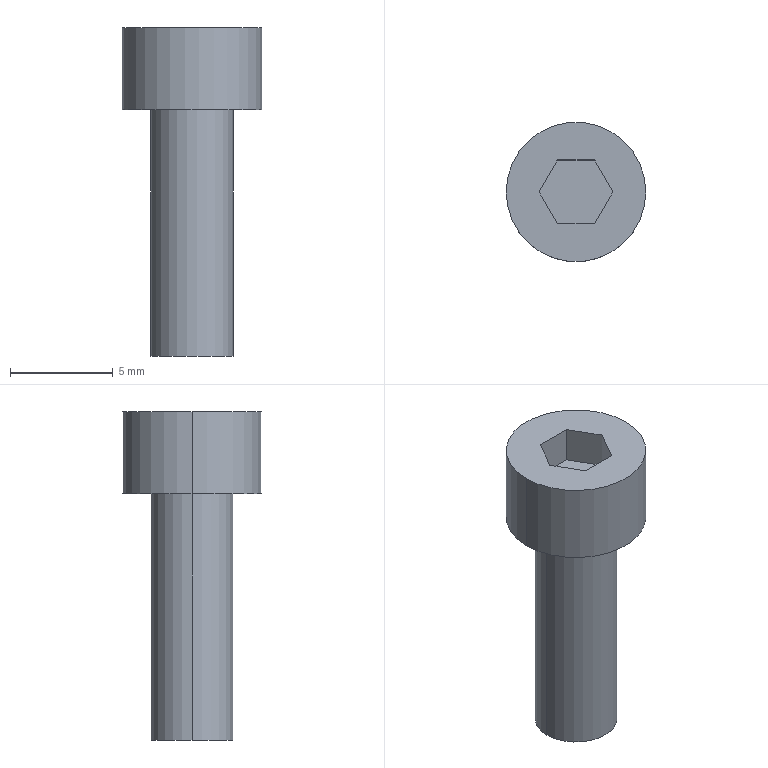Part | SolidWorks | features BaseBody 1 | 1 solid | 14 faces | box 6.8 x 6.8 x 16 mm | volume 280.912 mm3 | plane 10 | cylinder 4 | commonest cylinder face diameters 4 x2 6.8 x2
STEP:
#1=CARTESIAN_POINT('',(2.,0.,-12.));
#2=VERTEX_POINT('',#1);
#3=CARTESIAN_POINT('',(-2.,0.,-12.));
#4=VERTEX_POINT('',#3);
#5=CARTESIAN_POINT('',(0.,0.,-12.));
#6=DIRECTION('',(0.,0.,1.));
#7=DIRECTION('',(1.,0.,0.));
#8=AXIS2_PLACEMENT_3D('',#5,#6,#7);
#9=CIRCLE('',#8,2.);
#10=EDGE_CURVE('',#2,#4,#9,.T.);
#11=ORIENTED_EDGE('',*,*,#10,.T.);
#12=CARTESIAN_POINT('',(-2.,0.,0.));
#13=VERTEX_POINT('',#12);
#14=CARTESIAN_POINT('',(-2.,0.,-12.));
#15=DIRECTION('',(0.,0.,1.));
#16=VECTOR('',#15,1000.);
#17=LINE('',#14,#16);
#18=EDGE_CURVE('',#4,#13,#17,.T.);
#19=ORIENTED_EDGE('',*,*,#18,.T.);
#20=CARTESIAN_POINT('',(2.,0.,0.));
#21=VERTEX_POINT('',#20);
#22=CARTESIAN_POINT('',(0.,0.,0.));
#23=DIRECTION('',(0.,0.,-1.));
#24=DIRECTION('',(1.,0.,0.));
#25=AXIS2_PLACEMENT_3D('',#22,#23,#24);
#26=CIRCLE('',#25,2.);
#27=EDGE_CURVE('',#13,#21,#26,.T.);
#28=ORIENTED_EDGE('',*,*,#27,.T.);
#29=CARTESIAN_POINT('',(2.,0.,-12.));
#30=DIRECTION('',(0.,0.,1.));
#31=VECTOR('',#30,1000.);
#32=LINE('',#29,#31);
#33=EDGE_CURVE('',#2,#21,#32,.T.);
#34=ORIENTED_EDGE('',*,*,#33,.F.);
#35=EDGE_LOOP('',(#11,#19,#28,#34));
#36=FACE_OUTER_BOUND('',#35,.T.);
#37=CARTESIAN_POINT('',(0.,0.,-12.));
#38=DIRECTION('',(0.,0.,1.));
#39=DIRECTION('',(1.,0.,0.));
#40=AXIS2_PLACEMENT_3D('',#37,#38,#39);
#41=CYLINDRICAL_SURFACE('',#40,2.);
#42=ADVANCED_FACE('',(#36),#41,.T.);
#43=CARTESIAN_POINT('',(3.4,0.,0.));
#44=VERTEX_POINT('',#43);
#45=CARTESIAN_POINT('',(-3.4,0.,0.));
#46=VERTEX_POINT('',#45);
#47=CARTESIAN_POINT('',(0.,0.,0.));
#48=DIRECTION('',(0.,0.,1.));
#49=DIRECTION('',(1.,0.,0.));
#50=AXIS2_PLACEMENT_3D('',#47,#48,#49);
#51=CIRCLE('',#50,3.4);
#52=EDGE_CURVE('',#44,#46,#51,.T.);
#53=ORIENTED_EDGE('',*,*,#52,.T.);
#54=CARTESIAN_POINT('',(-3.4,0.,4.));
#55=VERTEX_POINT('',#54);
#56=CARTESIAN_POINT('',(-3.4,0.,0.));
#57=DIRECTION('',(0.,0.,1.));
#58=VECTOR('',#57,1000.);
#59=LINE('',#56,#58);
#60=EDGE_CURVE('',#46,#55,#59,.T.);
#61=ORIENTED_EDGE('',*,*,#60,.T.);
#62=CARTESIAN_POINT('',(3.4,0.,4.));
#63=VERTEX_POINT('',#62);
#64=CARTESIAN_POINT('',(0.,0.,4.));
#65=DIRECTION('',(0.,0.,-1.));
#66=DIRECTION('',(1.,0.,0.));
#67=AXIS2_PLACEMENT_3D('',#64,#65,#66);
#68=CIRCLE('',#67,3.4);
#69=EDGE_CURVE('',#55,#63,#68,.T.);
#70=ORIENTED_EDGE('',*,*,#69,.T.);
#71=CARTESIAN_POINT('',(3.4,0.,0.));
#72=DIRECTION('',(0.,0.,1.));
#73=VECTOR('',#72,1000.);
#74=LINE('',#71,#73);
#75=EDGE_CURVE('',#44,#63,#74,.T.);
#76=ORIENTED_EDGE('',*,*,#75,.F.);
#77=EDGE_LOOP('',(#53,#61,#70,#76));
#78=FACE_OUTER_BOUND('',#77,.T.);
#79=CARTESIAN_POINT('',(0.,0.,0.));
#80=DIRECTION('',(0.,0.,1.));
#81=DIRECTION('',(1.,0.,0.));
#82=AXIS2_PLACEMENT_3D('',#79,#80,#81);
#83=CYLINDRICAL_SURFACE('',#82,3.4);
#84=ADVANCED_FACE('',(#78),#83,.T.);
#85=ORIENTED_EDGE('',*,*,#18,.F.);
#86=CARTESIAN_POINT('',(0.,0.,-12.));
#87=DIRECTION('',(0.,0.,1.));
#88=DIRECTION('',(1.,0.,0.));
#89=AXIS2_PLACEMENT_3D('',#86,#87,#88);
#90=CIRCLE('',#89,2.);
#91=EDGE_CURVE('',#4,#2,#90,.T.);
#92=ORIENTED_EDGE('',*,*,#91,.T.);
#93=ORIENTED_EDGE('',*,*,#33,.T.);
#94=CARTESIAN_POINT('',(0.,0.,0.));
#95=DIRECTION('',(0.,0.,-1.));
#96=DIRECTION('',(1.,0.,0.));
#97=AXIS2_PLACEMENT_3D('',#94,#95,#96);
#98=CIRCLE('',#97,2.);
#99=EDGE_CURVE('',#21,#13,#98,.T.);
#100=ORIENTED_EDGE('',*,*,#99,.T.);
#101=EDGE_LOOP('',(#85,#92,#93,#100));
#102=FACE_OUTER_BOUND('',#101,.T.);
#103=CARTESIAN_POINT('',(0.,0.,-12.));
#104=DIRECTION('',(0.,0.,1.));
#105=DIRECTION('',(1.,0.,0.));
#106=AXIS2_PLACEMENT_3D('',#103,#104,#105);
#107=CYLINDRICAL_SURFACE('',#106,2.);
#108=ADVANCED_FACE('',(#102),#107,.T.);
#109=ORIENTED_EDGE('',*,*,#10,.F.);
#110=ORIENTED_EDGE('',*,*,#91,.F.);
#111=EDGE_LOOP('',(#109,#110));
#112=FACE_OUTER_BOUND('',#111,.T.);
#113=CARTESIAN_POINT('',(0.,0.,-12.));
#114=DIRECTION('',(0.,0.,1.));
#115=DIRECTION('',(1.,0.,0.));
#116=AXIS2_PLACEMENT_3D('',#113,#114,#115);
#117=PLANE('',#116);
#118=ADVANCED_FACE('',(#112),#117,.F.);
#119=ORIENTED_EDGE('',*,*,#99,.F.);
#120=ORIENTED_EDGE('',*,*,#27,.F.);
#121=EDGE_LOOP('',(#119,#120));
#122=FACE_BOUND('',#121,.T.);
#123=ORIENTED_EDGE('',*,*,#52,.F.);
#124=CARTESIAN_POINT('',(0.,0.,0.));
#125=DIRECTION('',(0.,0.,1.));
#126=DIRECTION('',(1.,0.,0.));
#127=AXIS2_PLACEMENT_3D('',#124,#125,#126);
#128=CIRCLE('',#127,3.4);
#129=EDGE_CURVE('',#46,#44,#128,.T.);
#130=ORIENTED_EDGE('',*,*,#129,.F.);
#131=EDGE_LOOP('',(#123,#130));
#132=FACE_OUTER_BOUND('',#131,.T.);
#133=CARTESIAN_POINT('',(0.,0.,0.));
#134=DIRECTION('',(0.,0.,1.));
#135=DIRECTION('',(1.,0.,0.));
#136=AXIS2_PLACEMENT_3D('',#133,#134,#135);
#137=PLANE('',#136);
#138=ADVANCED_FACE('',(#122,#132),#137,.F.);
#139=ORIENTED_EDGE('',*,*,#60,.F.);
#140=ORIENTED_EDGE('',*,*,#129,.T.);
#141=ORIENTED_EDGE('',*,*,#75,.T.);
#142=CARTESIAN_POINT('',(0.,0.,4.));
#143=DIRECTION('',(0.,0.,-1.));
#144=DIRECTION('',(1.,0.,0.));
#145=AXIS2_PLACEMENT_3D('',#142,#143,#144);
#146=CIRCLE('',#145,3.4);
#147=EDGE_CURVE('',#63,#55,#146,.T.);
#148=ORIENTED_EDGE('',*,*,#147,.T.);
#149=EDGE_LOOP('',(#139,#140,#141,#148));
#150=FACE_OUTER_BOUND('',#149,.T.);
#151=CARTESIAN_POINT('',(0.,0.,0.));
#152=DIRECTION('',(0.,0.,1.));
#153=DIRECTION('',(1.,0.,0.));
#154=AXIS2_PLACEMENT_3D('',#151,#152,#153);
#155=CYLINDRICAL_SURFACE('',#154,3.4);
#156=ADVANCED_FACE('',(#150),#155,.T.);
#157=CARTESIAN_POINT('',(-0.9,-1.559,4.));
#158=VERTEX_POINT('',#157);
#159=CARTESIAN_POINT('',(-1.8,0.,4.));
#160=VERTEX_POINT('',#159);
#161=CARTESIAN_POINT('',(-0.9,-1.559,4.));
#162=DIRECTION('',(-0.5,0.866,0.));
#163=VECTOR('',#162,1000.);
#164=LINE('',#161,#163);
#165=EDGE_CURVE('',#158,#160,#164,.T.);
#166=ORIENTED_EDGE('',*,*,#165,.T.);
#167=CARTESIAN_POINT('',(-0.9,1.559,4.));
#168=VERTEX_POINT('',#167);
#169=CARTESIAN_POINT('',(-1.8,0.,4.));
#170=DIRECTION('',(0.5,0.866,0.));
#171=VECTOR('',#170,1000.);
#172=LINE('',#169,#171);
#173=EDGE_CURVE('',#160,#168,#172,.T.);
#174=ORIENTED_EDGE('',*,*,#173,.T.);
#175=CARTESIAN_POINT('',(0.9,1.559,4.));
#176=VERTEX_POINT('',#175);
#177=CARTESIAN_POINT('',(0.,1.559,4.));
#178=DIRECTION('',(1.,0.,0.));
#179=VECTOR('',#178,1000.);
#180=LINE('',#177,#179);
#181=EDGE_CURVE('',#168,#176,#180,.T.);
#182=ORIENTED_EDGE('',*,*,#181,.T.);
#183=CARTESIAN_POINT('',(1.8,0.,4.));
#184=VERTEX_POINT('',#183);
#185=CARTESIAN_POINT('',(0.9,1.559,4.));
#186=DIRECTION('',(0.5,-0.866,0.));
#187=VECTOR('',#186,1000.);
#188=LINE('',#185,#187);
#189=EDGE_CURVE('',#176,#184,#188,.T.);
#190=ORIENTED_EDGE('',*,*,#189,.T.);
#191=CARTESIAN_POINT('',(0.9,-1.559,4.));
#192=VERTEX_POINT('',#191);
#193=CARTESIAN_POINT('',(1.8,0.,4.));
#194=DIRECTION('',(-0.5,-0.866,0.));
#195=VECTOR('',#194,1000.);
#196=LINE('',#193,#195);
#197=EDGE_CURVE('',#184,#192,#196,.T.);
#198=ORIENTED_EDGE('',*,*,#197,.T.);
#199=CARTESIAN_POINT('',(0.,-1.559,4.));
#200=DIRECTION('',(-1.,0.,0.));
#201=VECTOR('',#200,1000.);
#202=LINE('',#199,#201);
#203=EDGE_CURVE('',#192,#158,#202,.T.);
#204=ORIENTED_EDGE('',*,*,#203,.T.);
#205=EDGE_LOOP('',(#166,#174,#182,#190,#198,#204));
#206=FACE_BOUND('',#205,.T.);
#207=ORIENTED_EDGE('',*,*,#147,.F.);
#208=ORIENTED_EDGE('',*,*,#69,.F.);
#209=EDGE_LOOP('',(#207,#208));
#210=FACE_OUTER_BOUND('',#209,.T.);
#211=CARTESIAN_POINT('',(0.,0.,4.));
#212=DIRECTION('',(0.,0.,1.));
#213=DIRECTION('',(1.,0.,0.));
#214=AXIS2_PLACEMENT_3D('',#211,#212,#213);
#215=PLANE('',#214);
#216=ADVANCED_FACE('',(#206,#210),#215,.T.);
#217=ORIENTED_EDGE('',*,*,#173,.F.);
#218=CARTESIAN_POINT('',(-1.8,0.,2.2));
#219=VERTEX_POINT('',#218);
#220=CARTESIAN_POINT('',(-1.8,0.,2.2));
#221=DIRECTION('',(0.,0.,-1.));
#222=VECTOR('',#221,1000.);
#223=LINE('',#220,#222);
#224=EDGE_CURVE('',#160,#219,#223,.T.);
#225=ORIENTED_EDGE('',*,*,#224,.T.);
#226=CARTESIAN_POINT('',(-0.9,1.559,2.2));
#227=VERTEX_POINT('',#226);
#228=CARTESIAN_POINT('',(-0.9,1.559,2.2));
#229=DIRECTION('',(0.5,0.866,0.));
#230=VECTOR('',#229,1000.);
#231=LINE('',#228,#230);
#232=EDGE_CURVE('',#219,#227,#231,.T.);
#233=ORIENTED_EDGE('',*,*,#232,.T.);
#234=CARTESIAN_POINT('',(-0.9,1.559,2.2));
#235=DIRECTION('',(0.,0.,1.));
#236=VECTOR('',#235,1000.);
#237=LINE('',#234,#236);
#238=EDGE_CURVE('',#227,#168,#237,.T.);
#239=ORIENTED_EDGE('',*,*,#238,.T.);
#240=EDGE_LOOP('',(#217,#225,#233,#239));
#241=FACE_OUTER_BOUND('',#240,.T.);
#242=CARTESIAN_POINT('',(-0.9,1.559,2.2));
#243=DIRECTION('',(0.866,-0.5,0.));
#244=DIRECTION('',(0.5,0.866,0.));
#245=AXIS2_PLACEMENT_3D('',#242,#243,#244);
#246=PLANE('',#245);
#247=ADVANCED_FACE('',(#241),#246,.T.);
#248=ORIENTED_EDGE('',*,*,#165,.F.);
#249=CARTESIAN_POINT('',(-0.9,-1.559,2.2));
#250=VERTEX_POINT('',#249);
#251=CARTESIAN_POINT('',(-0.9,-1.559,2.2));
#252=DIRECTION('',(0.,0.,-1.));
#253=VECTOR('',#252,1000.);
#254=LINE('',#251,#253);
#255=EDGE_CURVE('',#158,#250,#254,.T.);
#256=ORIENTED_EDGE('',*,*,#255,.T.);
#257=CARTESIAN_POINT('',(-1.8,0.,2.2));
#258=DIRECTION('',(-0.5,0.866,0.));
#259=VECTOR('',#258,1000.);
#260=LINE('',#257,#259);
#261=EDGE_CURVE('',#250,#219,#260,.T.);
#262=ORIENTED_EDGE('',*,*,#261,.T.);
#263=ORIENTED_EDGE('',*,*,#224,.F.);
#264=EDGE_LOOP('',(#248,#256,#262,#263));
#265=FACE_OUTER_BOUND('',#264,.T.);
#266=CARTESIAN_POINT('',(-1.8,0.,2.2));
#267=DIRECTION('',(0.866,0.5,0.));
#268=DIRECTION('',(-0.5,0.866,0.));
#269=AXIS2_PLACEMENT_3D('',#266,#267,#268);
#270=PLANE('',#269);
#271=ADVANCED_FACE('',(#265),#270,.T.);
#272=ORIENTED_EDGE('',*,*,#203,.F.);
#273=CARTESIAN_POINT('',(0.9,-1.559,2.2));
#274=VERTEX_POINT('',#273);
#275=CARTESIAN_POINT('',(0.9,-1.559,2.2));
#276=DIRECTION('',(0.,0.,-1.));
#277=VECTOR('',#276,1000.);
#278=LINE('',#275,#277);
#279=EDGE_CURVE('',#192,#274,#278,.T.);
#280=ORIENTED_EDGE('',*,*,#279,.T.);
#281=CARTESIAN_POINT('',(-0.9,-1.559,2.2));
#282=DIRECTION('',(-1.,0.,0.));
#283=VECTOR('',#282,1000.);
#284=LINE('',#281,#283);
#285=EDGE_CURVE('',#274,#250,#284,.T.);
#286=ORIENTED_EDGE('',*,*,#285,.T.);
#287=ORIENTED_EDGE('',*,*,#255,.F.);
#288=EDGE_LOOP('',(#272,#280,#286,#287));
#289=FACE_OUTER_BOUND('',#288,.T.);
#290=CARTESIAN_POINT('',(-0.9,-1.559,2.2));
#291=DIRECTION('',(0.,1.,0.));
#292=DIRECTION('',(-1.,0.,0.));
#293=AXIS2_PLACEMENT_3D('',#290,#291,#292);
#294=PLANE('',#293);
#295=ADVANCED_FACE('',(#289),#294,.T.);
#296=ORIENTED_EDGE('',*,*,#197,.F.);
#297=CARTESIAN_POINT('',(1.8,0.,2.2));
#298=VERTEX_POINT('',#297);
#299=CARTESIAN_POINT('',(1.8,0.,2.2));
#300=DIRECTION('',(0.,0.,-1.));
#301=VECTOR('',#300,1000.);
#302=LINE('',#299,#301);
#303=EDGE_CURVE('',#184,#298,#302,.T.);
#304=ORIENTED_EDGE('',*,*,#303,.T.);
#305=CARTESIAN_POINT('',(0.9,-1.559,2.2));
#306=DIRECTION('',(-0.5,-0.866,0.));
#307=VECTOR('',#306,1000.);
#308=LINE('',#305,#307);
#309=EDGE_CURVE('',#298,#274,#308,.T.);
#310=ORIENTED_EDGE('',*,*,#309,.T.);
#311=ORIENTED_EDGE('',*,*,#279,.F.);
#312=EDGE_LOOP('',(#296,#304,#310,#311));
#313=FACE_OUTER_BOUND('',#312,.T.);
#314=CARTESIAN_POINT('',(0.9,-1.559,2.2));
#315=DIRECTION('',(-0.866,0.5,0.));
#316=DIRECTION('',(-0.5,-0.866,0.));
#317=AXIS2_PLACEMENT_3D('',#314,#315,#316);
#318=PLANE('',#317);
#319=ADVANCED_FACE('',(#313),#318,.T.);
#320=ORIENTED_EDGE('',*,*,#189,.F.);
#321=CARTESIAN_POINT('',(0.9,1.559,2.2));
#322=VERTEX_POINT('',#321);
#323=CARTESIAN_POINT('',(0.9,1.559,2.2));
#324=DIRECTION('',(0.,0.,-1.));
#325=VECTOR('',#324,1000.);
#326=LINE('',#323,#325);
#327=EDGE_CURVE('',#176,#322,#326,.T.);
#328=ORIENTED_EDGE('',*,*,#327,.T.);
#329=CARTESIAN_POINT('',(1.8,0.,2.2));
#330=DIRECTION('',(0.5,-0.866,0.));
#331=VECTOR('',#330,1000.);
#332=LINE('',#329,#331);
#333=EDGE_CURVE('',#322,#298,#332,.T.);
#334=ORIENTED_EDGE('',*,*,#333,.T.);
#335=ORIENTED_EDGE('',*,*,#303,.F.);
#336=EDGE_LOOP('',(#320,#328,#334,#335));
#337=FACE_OUTER_BOUND('',#336,.T.);
#338=CARTESIAN_POINT('',(1.8,0.,2.2));
#339=DIRECTION('',(-0.866,-0.5,0.));
#340=DIRECTION('',(0.5,-0.866,0.));
#341=AXIS2_PLACEMENT_3D('',#338,#339,#340);
#342=PLANE('',#341);
#343=ADVANCED_FACE('',(#337),#342,.T.);
#344=ORIENTED_EDGE('',*,*,#181,.F.);
#345=ORIENTED_EDGE('',*,*,#238,.F.);
#346=CARTESIAN_POINT('',(0.9,1.559,2.2));
#347=DIRECTION('',(1.,0.,0.));
#348=VECTOR('',#347,1000.);
#349=LINE('',#346,#348);
#350=EDGE_CURVE('',#227,#322,#349,.T.);
#351=ORIENTED_EDGE('',*,*,#350,.T.);
#352=ORIENTED_EDGE('',*,*,#327,.F.);
#353=EDGE_LOOP('',(#344,#345,#351,#352));
#354=FACE_OUTER_BOUND('',#353,.T.);
#355=CARTESIAN_POINT('',(0.9,1.559,2.2));
#356=DIRECTION('',(0.,-1.,0.));
#357=DIRECTION('',(1.,0.,0.));
#358=AXIS2_PLACEMENT_3D('',#355,#356,#357);
#359=PLANE('',#358);
#360=ADVANCED_FACE('',(#354),#359,.T.);
#361=ORIENTED_EDGE('',*,*,#285,.F.);
#362=ORIENTED_EDGE('',*,*,#309,.F.);
#363=ORIENTED_EDGE('',*,*,#333,.F.);
#364=ORIENTED_EDGE('',*,*,#350,.F.);
#365=ORIENTED_EDGE('',*,*,#232,.F.);
#366=ORIENTED_EDGE('',*,*,#261,.F.);
#367=EDGE_LOOP('',(#361,#362,#363,#364,#365,#366));
#368=FACE_OUTER_BOUND('',#367,.T.);
#369=CARTESIAN_POINT('',(0.,0.,2.2));
#370=DIRECTION('',(0.,0.,1.));
#371=DIRECTION('',(1.,0.,0.));
#372=AXIS2_PLACEMENT_3D('',#369,#370,#371);
#373=PLANE('',#372);
#374=ADVANCED_FACE('',(#368),#373,.T.);
#375=CLOSED_SHELL('',(#42,#84,#108,#118,#138,#156,#216,#247,#271,#295,#319,#343,#360,#374));
#376=MANIFOLD_SOLID_BREP('',#375);
#377=CARTESIAN_POINT('',(0.,0.,0.));
#378=DIRECTION('',(0.,0.,1.));
#379=DIRECTION('',(1.,0.,0.));
#380=AXIS2_PLACEMENT_3D('',#377,#378,#379);
#381=(LENGTH_UNIT()NAMED_UNIT(*)SI_UNIT(.MILLI.,.METRE.));
#382=UNCERTAINTY_MEASURE_WITH_UNIT(LENGTH_MEASURE(0.00001),#381,'','');
#383=(NAMED_UNIT(*)PLANE_ANGLE_UNIT()SI_UNIT($,.RADIAN.));
#384=(NAMED_UNIT(*)SI_UNIT($,.STERADIAN.)SOLID_ANGLE_UNIT());
#385=(GEOMETRIC_REPRESENTATION_CONTEXT(3)GLOBAL_UNCERTAINTY_ASSIGNED_CONTEXT((#382))GLOBAL_UNIT_ASSIGNED_CONTEXT((#381,#383,#384))REPRESENTATION_CONTEXT('',''));
#386=ADVANCED_BREP_SHAPE_REPRESENTATION('',(#376,#380),#385);